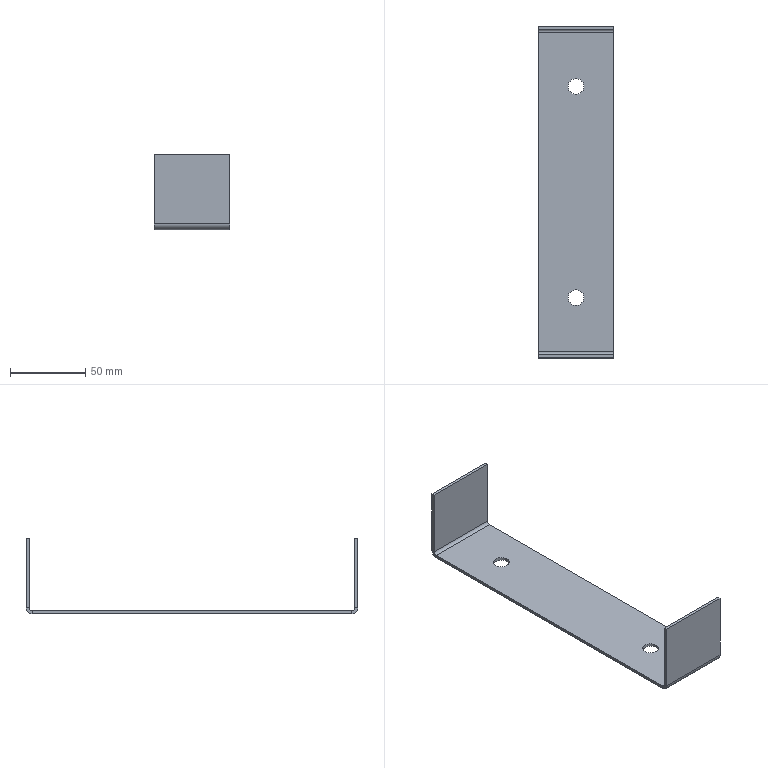Part | STEP file | SYL_0392D6J1SYL0380DJ100-674343 | 1 solid | 26 faces | box 50 x 220 x 50 mm | volume 30996 mm3 | plane 18 | cylinder 8 | commonest cylinder face diameters 10.5 x4 4 x2 8 x2
STEP:
#1=CARTESIAN_POINT('',(5.25,70.,-25.));
#2=VERTEX_POINT('',#1);
#3=CARTESIAN_POINT('',(5.25,70.,-23.));
#4=VERTEX_POINT('',#3);
#5=CARTESIAN_POINT('',(5.25,70.,-23.));
#6=DIRECTION('',(0.,0.,1.));
#7=VECTOR('',#6,1000.);
#8=LINE('',#5,#7);
#9=EDGE_CURVE('',#2,#4,#8,.T.);
#10=ORIENTED_EDGE('',*,*,#9,.F.);
#11=CARTESIAN_POINT('',(-5.25,70.,-25.));
#12=VERTEX_POINT('',#11);
#13=CARTESIAN_POINT('',(0.,70.,-25.));
#14=DIRECTION('',(0.,0.,-1.));
#15=DIRECTION('',(-1.,0.,0.));
#16=AXIS2_PLACEMENT_3D('',#13,#14,#15);
#17=CIRCLE('',#16,5.25);
#18=EDGE_CURVE('',#2,#12,#17,.T.);
#19=ORIENTED_EDGE('',*,*,#18,.T.);
#20=CARTESIAN_POINT('',(-5.25,70.,-23.));
#21=VERTEX_POINT('',#20);
#22=CARTESIAN_POINT('',(-5.25,70.,-23.));
#23=DIRECTION('',(0.,0.,1.));
#24=VECTOR('',#23,1000.);
#25=LINE('',#22,#24);
#26=EDGE_CURVE('',#12,#21,#25,.T.);
#27=ORIENTED_EDGE('',*,*,#26,.T.);
#28=CARTESIAN_POINT('',(0.,70.,-23.));
#29=DIRECTION('',(0.,0.,-1.));
#30=DIRECTION('',(1.,0.,0.));
#31=AXIS2_PLACEMENT_3D('',#28,#29,#30);
#32=CIRCLE('',#31,5.25);
#33=EDGE_CURVE('',#4,#21,#32,.T.);
#34=ORIENTED_EDGE('',*,*,#33,.F.);
#35=EDGE_LOOP('',(#10,#19,#27,#34));
#36=FACE_OUTER_BOUND('',#35,.T.);
#37=CARTESIAN_POINT('',(0.,70.,-23.));
#38=DIRECTION('',(0.,0.,-1.));
#39=DIRECTION('',(-1.,0.,0.));
#40=AXIS2_PLACEMENT_3D('',#37,#38,#39);
#41=CYLINDRICAL_SURFACE('',#40,5.25);
#42=ADVANCED_FACE('',(#36),#41,.F.);
#43=CARTESIAN_POINT('',(5.25,-70.,-25.));
#44=VERTEX_POINT('',#43);
#45=CARTESIAN_POINT('',(5.25,-70.,-23.));
#46=VERTEX_POINT('',#45);
#47=CARTESIAN_POINT('',(5.25,-70.,-23.));
#48=DIRECTION('',(0.,0.,1.));
#49=VECTOR('',#48,1000.);
#50=LINE('',#47,#49);
#51=EDGE_CURVE('',#44,#46,#50,.T.);
#52=ORIENTED_EDGE('',*,*,#51,.F.);
#53=CARTESIAN_POINT('',(-5.25,-70.,-25.));
#54=VERTEX_POINT('',#53);
#55=CARTESIAN_POINT('',(0.,-70.,-25.));
#56=DIRECTION('',(0.,0.,-1.));
#57=DIRECTION('',(-1.,0.,0.));
#58=AXIS2_PLACEMENT_3D('',#55,#56,#57);
#59=CIRCLE('',#58,5.25);
#60=EDGE_CURVE('',#44,#54,#59,.T.);
#61=ORIENTED_EDGE('',*,*,#60,.T.);
#62=CARTESIAN_POINT('',(-5.25,-70.,-23.));
#63=VERTEX_POINT('',#62);
#64=CARTESIAN_POINT('',(-5.25,-70.,-23.));
#65=DIRECTION('',(0.,0.,1.));
#66=VECTOR('',#65,1000.);
#67=LINE('',#64,#66);
#68=EDGE_CURVE('',#54,#63,#67,.T.);
#69=ORIENTED_EDGE('',*,*,#68,.T.);
#70=CARTESIAN_POINT('',(0.,-70.,-23.));
#71=DIRECTION('',(0.,0.,-1.));
#72=DIRECTION('',(1.,0.,0.));
#73=AXIS2_PLACEMENT_3D('',#70,#71,#72);
#74=CIRCLE('',#73,5.25);
#75=EDGE_CURVE('',#46,#63,#74,.T.);
#76=ORIENTED_EDGE('',*,*,#75,.F.);
#77=EDGE_LOOP('',(#52,#61,#69,#76));
#78=FACE_OUTER_BOUND('',#77,.T.);
#79=CARTESIAN_POINT('',(0.,-70.,-23.));
#80=DIRECTION('',(0.,0.,-1.));
#81=DIRECTION('',(-1.,0.,0.));
#82=AXIS2_PLACEMENT_3D('',#79,#80,#81);
#83=CYLINDRICAL_SURFACE('',#82,5.25);
#84=ADVANCED_FACE('',(#78),#83,.F.);
#85=CARTESIAN_POINT('',(25.,106.,-25.));
#86=VERTEX_POINT('',#85);
#87=CARTESIAN_POINT('',(25.,106.,-23.));
#88=VERTEX_POINT('',#87);
#89=CARTESIAN_POINT('',(25.,106.,-23.));
#90=DIRECTION('',(0.,0.,1.));
#91=VECTOR('',#90,1000.);
#92=LINE('',#89,#91);
#93=EDGE_CURVE('',#86,#88,#92,.T.);
#94=ORIENTED_EDGE('',*,*,#93,.F.);
#95=CARTESIAN_POINT('',(25.,110.,-21.));
#96=VERTEX_POINT('',#95);
#97=CARTESIAN_POINT('',(25.,106.,-21.));
#98=DIRECTION('',(-1.,0.,0.));
#99=DIRECTION('',(0.,0.,1.));
#100=AXIS2_PLACEMENT_3D('',#97,#98,#99);
#101=CIRCLE('',#100,4.);
#102=EDGE_CURVE('',#96,#86,#101,.T.);
#103=ORIENTED_EDGE('',*,*,#102,.F.);
#104=CARTESIAN_POINT('',(25.,108.,-21.));
#105=VERTEX_POINT('',#104);
#106=CARTESIAN_POINT('',(25.,108.,-21.));
#107=DIRECTION('',(0.,-1.,0.));
#108=VECTOR('',#107,1000.);
#109=LINE('',#106,#108);
#110=EDGE_CURVE('',#96,#105,#109,.T.);
#111=ORIENTED_EDGE('',*,*,#110,.T.);
#112=CARTESIAN_POINT('',(25.,106.,-21.));
#113=DIRECTION('',(-1.,0.,0.));
#114=DIRECTION('',(0.,1.,0.));
#115=AXIS2_PLACEMENT_3D('',#112,#113,#114);
#116=CIRCLE('',#115,2.);
#117=EDGE_CURVE('',#105,#88,#116,.T.);
#118=ORIENTED_EDGE('',*,*,#117,.T.);
#119=EDGE_LOOP('',(#94,#103,#111,#118));
#120=FACE_OUTER_BOUND('',#119,.T.);
#121=CARTESIAN_POINT('',(25.,106.,-21.));
#122=DIRECTION('',(1.,0.,0.));
#123=DIRECTION('',(0.,0.,-1.));
#124=AXIS2_PLACEMENT_3D('',#121,#122,#123);
#125=PLANE('',#124);
#126=ADVANCED_FACE('',(#120),#125,.T.);
#127=ORIENTED_EDGE('',*,*,#110,.F.);
#128=CARTESIAN_POINT('',(25.,110.,25.));
#129=VERTEX_POINT('',#128);
#130=CARTESIAN_POINT('',(25.,110.,-25.));
#131=DIRECTION('',(0.,0.,-1.));
#132=VECTOR('',#131,1000.);
#133=LINE('',#130,#132);
#134=EDGE_CURVE('',#129,#96,#133,.T.);
#135=ORIENTED_EDGE('',*,*,#134,.F.);
#136=CARTESIAN_POINT('',(25.,108.,25.));
#137=VERTEX_POINT('',#136);
#138=CARTESIAN_POINT('',(25.,108.,25.));
#139=DIRECTION('',(0.,-1.,0.));
#140=VECTOR('',#139,1000.);
#141=LINE('',#138,#140);
#142=EDGE_CURVE('',#129,#137,#141,.T.);
#143=ORIENTED_EDGE('',*,*,#142,.T.);
#144=CARTESIAN_POINT('',(25.,108.,25.));
#145=DIRECTION('',(0.,0.,-1.));
#146=VECTOR('',#145,1000.);
#147=LINE('',#144,#146);
#148=EDGE_CURVE('',#137,#105,#147,.T.);
#149=ORIENTED_EDGE('',*,*,#148,.T.);
#150=EDGE_LOOP('',(#127,#135,#143,#149));
#151=FACE_OUTER_BOUND('',#150,.T.);
#152=CARTESIAN_POINT('',(25.,108.,25.));
#153=DIRECTION('',(1.,0.,0.));
#154=DIRECTION('',(0.,0.,-1.));
#155=AXIS2_PLACEMENT_3D('',#152,#153,#154);
#156=PLANE('',#155);
#157=ADVANCED_FACE('',(#151),#156,.T.);
#158=ORIENTED_EDGE('',*,*,#142,.F.);
#159=CARTESIAN_POINT('',(-25.,110.,25.));
#160=VERTEX_POINT('',#159);
#161=CARTESIAN_POINT('',(-25.,110.,25.));
#162=DIRECTION('',(-1.,0.,0.));
#163=VECTOR('',#162,1000.);
#164=LINE('',#161,#163);
#165=EDGE_CURVE('',#129,#160,#164,.T.);
#166=ORIENTED_EDGE('',*,*,#165,.T.);
#167=CARTESIAN_POINT('',(-25.,108.,25.));
#168=VERTEX_POINT('',#167);
#169=CARTESIAN_POINT('',(-25.,108.,25.));
#170=DIRECTION('',(0.,-1.,0.));
#171=VECTOR('',#170,1000.);
#172=LINE('',#169,#171);
#173=EDGE_CURVE('',#160,#168,#172,.T.);
#174=ORIENTED_EDGE('',*,*,#173,.T.);
#175=CARTESIAN_POINT('',(25.,108.,25.));
#176=DIRECTION('',(-1.,0.,0.));
#177=VECTOR('',#176,1000.);
#178=LINE('',#175,#177);
#179=EDGE_CURVE('',#137,#168,#178,.T.);
#180=ORIENTED_EDGE('',*,*,#179,.F.);
#181=EDGE_LOOP('',(#158,#166,#174,#180));
#182=FACE_OUTER_BOUND('',#181,.T.);
#183=CARTESIAN_POINT('',(25.,108.,25.));
#184=DIRECTION('',(0.,0.,-1.));
#185=DIRECTION('',(-1.,0.,0.));
#186=AXIS2_PLACEMENT_3D('',#183,#184,#185);
#187=PLANE('',#186);
#188=ADVANCED_FACE('',(#182),#187,.F.);
#189=ORIENTED_EDGE('',*,*,#173,.F.);
#190=CARTESIAN_POINT('',(-25.,110.,-21.));
#191=VERTEX_POINT('',#190);
#192=CARTESIAN_POINT('',(-25.,110.,-25.));
#193=DIRECTION('',(0.,0.,-1.));
#194=VECTOR('',#193,1000.);
#195=LINE('',#192,#194);
#196=EDGE_CURVE('',#160,#191,#195,.T.);
#197=ORIENTED_EDGE('',*,*,#196,.T.);
#198=CARTESIAN_POINT('',(-25.,108.,-21.));
#199=VERTEX_POINT('',#198);
#200=CARTESIAN_POINT('',(-25.,108.,-21.));
#201=DIRECTION('',(0.,-1.,0.));
#202=VECTOR('',#201,1000.);
#203=LINE('',#200,#202);
#204=EDGE_CURVE('',#191,#199,#203,.T.);
#205=ORIENTED_EDGE('',*,*,#204,.T.);
#206=CARTESIAN_POINT('',(-25.,108.,25.));
#207=DIRECTION('',(0.,0.,-1.));
#208=VECTOR('',#207,1000.);
#209=LINE('',#206,#208);
#210=EDGE_CURVE('',#168,#199,#209,.T.);
#211=ORIENTED_EDGE('',*,*,#210,.F.);
#212=EDGE_LOOP('',(#189,#197,#205,#211));
#213=FACE_OUTER_BOUND('',#212,.T.);
#214=CARTESIAN_POINT('',(-25.,108.,25.));
#215=DIRECTION('',(1.,0.,0.));
#216=DIRECTION('',(0.,0.,-1.));
#217=AXIS2_PLACEMENT_3D('',#214,#215,#216);
#218=PLANE('',#217);
#219=ADVANCED_FACE('',(#213),#218,.F.);
#220=ORIENTED_EDGE('',*,*,#204,.F.);
#221=CARTESIAN_POINT('',(-25.,106.,-25.));
#222=VERTEX_POINT('',#221);
#223=CARTESIAN_POINT('',(-25.,106.,-21.));
#224=DIRECTION('',(1.,0.,0.));
#225=DIRECTION('',(0.,0.,1.));
#226=AXIS2_PLACEMENT_3D('',#223,#224,#225);
#227=CIRCLE('',#226,4.);
#228=EDGE_CURVE('',#222,#191,#227,.T.);
#229=ORIENTED_EDGE('',*,*,#228,.F.);
#230=CARTESIAN_POINT('',(-25.,106.,-23.));
#231=VERTEX_POINT('',#230);
#232=CARTESIAN_POINT('',(-25.,106.,-23.));
#233=DIRECTION('',(0.,0.,1.));
#234=VECTOR('',#233,1000.);
#235=LINE('',#232,#234);
#236=EDGE_CURVE('',#222,#231,#235,.T.);
#237=ORIENTED_EDGE('',*,*,#236,.T.);
#238=CARTESIAN_POINT('',(-25.,106.,-21.));
#239=DIRECTION('',(1.,0.,0.));
#240=DIRECTION('',(0.,0.,-1.));
#241=AXIS2_PLACEMENT_3D('',#238,#239,#240);
#242=CIRCLE('',#241,2.);
#243=EDGE_CURVE('',#231,#199,#242,.T.);
#244=ORIENTED_EDGE('',*,*,#243,.T.);
#245=EDGE_LOOP('',(#220,#229,#237,#244));
#246=FACE_OUTER_BOUND('',#245,.T.);
#247=CARTESIAN_POINT('',(-25.,106.,-21.));
#248=DIRECTION('',(-1.,0.,0.));
#249=DIRECTION('',(0.,0.,1.));
#250=AXIS2_PLACEMENT_3D('',#247,#248,#249);
#251=PLANE('',#250);
#252=ADVANCED_FACE('',(#246),#251,.T.);
#253=ORIENTED_EDGE('',*,*,#236,.F.);
#254=CARTESIAN_POINT('',(-25.,-106.,-25.));
#255=VERTEX_POINT('',#254);
#256=CARTESIAN_POINT('',(-25.,-110.,-25.));
#257=DIRECTION('',(0.,-1.,0.));
#258=VECTOR('',#257,1000.);
#259=LINE('',#256,#258);
#260=EDGE_CURVE('',#222,#255,#259,.T.);
#261=ORIENTED_EDGE('',*,*,#260,.T.);
#262=CARTESIAN_POINT('',(-25.,-106.,-23.));
#263=VERTEX_POINT('',#262);
#264=CARTESIAN_POINT('',(-25.,-106.,-23.));
#265=DIRECTION('',(0.,0.,1.));
#266=VECTOR('',#265,1000.);
#267=LINE('',#264,#266);
#268=EDGE_CURVE('',#255,#263,#267,.T.);
#269=ORIENTED_EDGE('',*,*,#268,.T.);
#270=CARTESIAN_POINT('',(-25.,106.,-23.));
#271=DIRECTION('',(0.,-1.,0.));
#272=VECTOR('',#271,1000.);
#273=LINE('',#270,#272);
#274=EDGE_CURVE('',#231,#263,#273,.T.);
#275=ORIENTED_EDGE('',*,*,#274,.F.);
#276=EDGE_LOOP('',(#253,#261,#269,#275));
#277=FACE_OUTER_BOUND('',#276,.T.);
#278=CARTESIAN_POINT('',(-25.,106.,-23.));
#279=DIRECTION('',(1.,0.,0.));
#280=DIRECTION('',(0.,-1.,0.));
#281=AXIS2_PLACEMENT_3D('',#278,#279,#280);
#282=PLANE('',#281);
#283=ADVANCED_FACE('',(#277),#282,.F.);
#284=ORIENTED_EDGE('',*,*,#268,.F.);
#285=CARTESIAN_POINT('',(-25.,-110.,-21.));
#286=VERTEX_POINT('',#285);
#287=CARTESIAN_POINT('',(-25.,-106.,-21.));
#288=DIRECTION('',(1.,0.,0.));
#289=DIRECTION('',(0.,0.,1.));
#290=AXIS2_PLACEMENT_3D('',#287,#288,#289);
#291=CIRCLE('',#290,4.);
#292=EDGE_CURVE('',#286,#255,#291,.T.);
#293=ORIENTED_EDGE('',*,*,#292,.F.);
#294=CARTESIAN_POINT('',(-25.,-108.,-21.));
#295=VERTEX_POINT('',#294);
#296=CARTESIAN_POINT('',(-25.,-108.,-21.));
#297=DIRECTION('',(0.,1.,0.));
#298=VECTOR('',#297,1000.);
#299=LINE('',#296,#298);
#300=EDGE_CURVE('',#286,#295,#299,.T.);
#301=ORIENTED_EDGE('',*,*,#300,.T.);
#302=CARTESIAN_POINT('',(-25.,-106.,-21.));
#303=DIRECTION('',(1.,0.,0.));
#304=DIRECTION('',(0.,-1.,0.));
#305=AXIS2_PLACEMENT_3D('',#302,#303,#304);
#306=CIRCLE('',#305,2.);
#307=EDGE_CURVE('',#295,#263,#306,.T.);
#308=ORIENTED_EDGE('',*,*,#307,.T.);
#309=EDGE_LOOP('',(#284,#293,#301,#308));
#310=FACE_OUTER_BOUND('',#309,.T.);
#311=CARTESIAN_POINT('',(-25.,-106.,-21.));
#312=DIRECTION('',(-1.,0.,0.));
#313=DIRECTION('',(0.,0.,1.));
#314=AXIS2_PLACEMENT_3D('',#311,#312,#313);
#315=PLANE('',#314);
#316=ADVANCED_FACE('',(#310),#315,.T.);
#317=ORIENTED_EDGE('',*,*,#300,.F.);
#318=CARTESIAN_POINT('',(-25.,-110.,25.));
#319=VERTEX_POINT('',#318);
#320=CARTESIAN_POINT('',(-25.,-110.,25.));
#321=DIRECTION('',(0.,0.,1.));
#322=VECTOR('',#321,1000.);
#323=LINE('',#320,#322);
#324=EDGE_CURVE('',#286,#319,#323,.T.);
#325=ORIENTED_EDGE('',*,*,#324,.T.);
#326=CARTESIAN_POINT('',(-25.,-108.,25.));
#327=VERTEX_POINT('',#326);
#328=CARTESIAN_POINT('',(-25.,-108.,25.));
#329=DIRECTION('',(0.,1.,0.));
#330=VECTOR('',#329,1000.);
#331=LINE('',#328,#330);
#332=EDGE_CURVE('',#319,#327,#331,.T.);
#333=ORIENTED_EDGE('',*,*,#332,.T.);
#334=CARTESIAN_POINT('',(-25.,-108.,-21.));
#335=DIRECTION('',(0.,0.,1.));
#336=VECTOR('',#335,1000.);
#337=LINE('',#334,#336);
#338=EDGE_CURVE('',#295,#327,#337,.T.);
#339=ORIENTED_EDGE('',*,*,#338,.F.);
#340=EDGE_LOOP('',(#317,#325,#333,#339));
#341=FACE_OUTER_BOUND('',#340,.T.);
#342=CARTESIAN_POINT('',(-25.,-108.,-21.));
#343=DIRECTION('',(1.,0.,0.));
#344=DIRECTION('',(0.,0.,1.));
#345=AXIS2_PLACEMENT_3D('',#342,#343,#344);
#346=PLANE('',#345);
#347=ADVANCED_FACE('',(#341),#346,.F.);
#348=ORIENTED_EDGE('',*,*,#332,.F.);
#349=CARTESIAN_POINT('',(25.,-110.,25.));
#350=VERTEX_POINT('',#349);
#351=CARTESIAN_POINT('',(-25.,-110.,25.));
#352=DIRECTION('',(-1.,0.,0.));
#353=VECTOR('',#352,1000.);
#354=LINE('',#351,#353);
#355=EDGE_CURVE('',#350,#319,#354,.T.);
#356=ORIENTED_EDGE('',*,*,#355,.F.);
#357=CARTESIAN_POINT('',(25.,-108.,25.));
#358=VERTEX_POINT('',#357);
#359=CARTESIAN_POINT('',(25.,-108.,25.));
#360=DIRECTION('',(0.,1.,0.));
#361=VECTOR('',#360,1000.);
#362=LINE('',#359,#361);
#363=EDGE_CURVE('',#350,#358,#362,.T.);
#364=ORIENTED_EDGE('',*,*,#363,.T.);
#365=CARTESIAN_POINT('',(25.,-108.,25.));
#366=DIRECTION('',(-1.,0.,0.));
#367=VECTOR('',#366,1000.);
#368=LINE('',#365,#367);
#369=EDGE_CURVE('',#358,#327,#368,.T.);
#370=ORIENTED_EDGE('',*,*,#369,.T.);
#371=EDGE_LOOP('',(#348,#356,#364,#370));
#372=FACE_OUTER_BOUND('',#371,.T.);
#373=CARTESIAN_POINT('',(25.,-108.,25.));
#374=DIRECTION('',(0.,0.,1.));
#375=DIRECTION('',(-1.,0.,0.));
#376=AXIS2_PLACEMENT_3D('',#373,#374,#375);
#377=PLANE('',#376);
#378=ADVANCED_FACE('',(#372),#377,.T.);
#379=ORIENTED_EDGE('',*,*,#363,.F.);
#380=CARTESIAN_POINT('',(25.,-110.,-21.));
#381=VERTEX_POINT('',#380);
#382=CARTESIAN_POINT('',(25.,-110.,25.));
#383=DIRECTION('',(0.,0.,1.));
#384=VECTOR('',#383,1000.);
#385=LINE('',#382,#384);
#386=EDGE_CURVE('',#381,#350,#385,.T.);
#387=ORIENTED_EDGE('',*,*,#386,.F.);
#388=CARTESIAN_POINT('',(25.,-108.,-21.));
#389=VERTEX_POINT('',#388);
#390=CARTESIAN_POINT('',(25.,-108.,-21.));
#391=DIRECTION('',(0.,1.,0.));
#392=VECTOR('',#391,1000.);
#393=LINE('',#390,#392);
#394=EDGE_CURVE('',#381,#389,#393,.T.);
#395=ORIENTED_EDGE('',*,*,#394,.T.);
#396=CARTESIAN_POINT('',(25.,-108.,-21.));
#397=DIRECTION('',(0.,0.,1.));
#398=VECTOR('',#397,1000.);
#399=LINE('',#396,#398);
#400=EDGE_CURVE('',#389,#358,#399,.T.);
#401=ORIENTED_EDGE('',*,*,#400,.T.);
#402=EDGE_LOOP('',(#379,#387,#395,#401));
#403=FACE_OUTER_BOUND('',#402,.T.);
#404=CARTESIAN_POINT('',(25.,-108.,-21.));
#405=DIRECTION('',(1.,0.,0.));
#406=DIRECTION('',(0.,0.,1.));
#407=AXIS2_PLACEMENT_3D('',#404,#405,#406);
#408=PLANE('',#407);
#409=ADVANCED_FACE('',(#403),#408,.T.);
#410=ORIENTED_EDGE('',*,*,#394,.F.);
#411=CARTESIAN_POINT('',(25.,-106.,-25.));
#412=VERTEX_POINT('',#411);
#413=CARTESIAN_POINT('',(25.,-106.,-21.));
#414=DIRECTION('',(-1.,0.,0.));
#415=DIRECTION('',(0.,0.,1.));
#416=AXIS2_PLACEMENT_3D('',#413,#414,#415);
#417=CIRCLE('',#416,4.);
#418=EDGE_CURVE('',#412,#381,#417,.T.);
#419=ORIENTED_EDGE('',*,*,#418,.F.);
#420=CARTESIAN_POINT('',(25.,-106.,-23.));
#421=VERTEX_POINT('',#420);
#422=CARTESIAN_POINT('',(25.,-106.,-23.));
#423=DIRECTION('',(0.,0.,1.));
#424=VECTOR('',#423,1000.);
#425=LINE('',#422,#424);
#426=EDGE_CURVE('',#412,#421,#425,.T.);
#427=ORIENTED_EDGE('',*,*,#426,.T.);
#428=CARTESIAN_POINT('',(25.,-106.,-21.));
#429=DIRECTION('',(-1.,0.,0.));
#430=DIRECTION('',(0.,0.,-1.));
#431=AXIS2_PLACEMENT_3D('',#428,#429,#430);
#432=CIRCLE('',#431,2.);
#433=EDGE_CURVE('',#421,#389,#432,.T.);
#434=ORIENTED_EDGE('',*,*,#433,.T.);
#435=EDGE_LOOP('',(#410,#419,#427,#434));
#436=FACE_OUTER_BOUND('',#435,.T.);
#437=CARTESIAN_POINT('',(25.,-106.,-21.));
#438=DIRECTION('',(1.,0.,0.));
#439=DIRECTION('',(0.,0.,-1.));
#440=AXIS2_PLACEMENT_3D('',#437,#438,#439);
#441=PLANE('',#440);
#442=ADVANCED_FACE('',(#436),#441,.T.);
#443=CARTESIAN_POINT('',(0.,-70.,-25.));
#444=DIRECTION('',(0.,0.,-1.));
#445=DIRECTION('',(-1.,0.,0.));
#446=AXIS2_PLACEMENT_3D('',#443,#444,#445);
#447=CIRCLE('',#446,5.25);
#448=EDGE_CURVE('',#54,#44,#447,.T.);
#449=ORIENTED_EDGE('',*,*,#448,.T.);
#450=ORIENTED_EDGE('',*,*,#51,.T.);
#451=CARTESIAN_POINT('',(0.,-70.,-23.));
#452=DIRECTION('',(0.,0.,-1.));
#453=DIRECTION('',(-1.,0.,0.));
#454=AXIS2_PLACEMENT_3D('',#451,#452,#453);
#455=CIRCLE('',#454,5.25);
#456=EDGE_CURVE('',#63,#46,#455,.T.);
#457=ORIENTED_EDGE('',*,*,#456,.F.);
#458=ORIENTED_EDGE('',*,*,#68,.F.);
#459=EDGE_LOOP('',(#449,#450,#457,#458));
#460=FACE_OUTER_BOUND('',#459,.T.);
#461=CARTESIAN_POINT('',(0.,-70.,-23.));
#462=DIRECTION('',(0.,0.,-1.));
#463=DIRECTION('',(-1.,0.,0.));
#464=AXIS2_PLACEMENT_3D('',#461,#462,#463);
#465=CYLINDRICAL_SURFACE('',#464,5.25);
#466=ADVANCED_FACE('',(#460),#465,.F.);
#467=CARTESIAN_POINT('',(0.,70.,-25.));
#468=DIRECTION('',(0.,0.,-1.));
#469=DIRECTION('',(-1.,0.,0.));
#470=AXIS2_PLACEMENT_3D('',#467,#468,#469);
#471=CIRCLE('',#470,5.25);
#472=EDGE_CURVE('',#12,#2,#471,.T.);
#473=ORIENTED_EDGE('',*,*,#472,.T.);
#474=ORIENTED_EDGE('',*,*,#9,.T.);
#475=CARTESIAN_POINT('',(0.,70.,-23.));
#476=DIRECTION('',(0.,0.,-1.));
#477=DIRECTION('',(-1.,0.,0.));
#478=AXIS2_PLACEMENT_3D('',#475,#476,#477);
#479=CIRCLE('',#478,5.25);
#480=EDGE_CURVE('',#21,#4,#479,.T.);
#481=ORIENTED_EDGE('',*,*,#480,.F.);
#482=ORIENTED_EDGE('',*,*,#26,.F.);
#483=EDGE_LOOP('',(#473,#474,#481,#482));
#484=FACE_OUTER_BOUND('',#483,.T.);
#485=CARTESIAN_POINT('',(0.,70.,-23.));
#486=DIRECTION('',(0.,0.,-1.));
#487=DIRECTION('',(-1.,0.,0.));
#488=AXIS2_PLACEMENT_3D('',#485,#486,#487);
#489=CYLINDRICAL_SURFACE('',#488,5.25);
#490=ADVANCED_FACE('',(#484),#489,.F.);
#491=CARTESIAN_POINT('',(25.,-110.,-25.));
#492=DIRECTION('',(0.,-1.,0.));
#493=VECTOR('',#492,1000.);
#494=LINE('',#491,#493);
#495=EDGE_CURVE('',#86,#412,#494,.T.);
#496=ORIENTED_EDGE('',*,*,#495,.F.);
#497=ORIENTED_EDGE('',*,*,#93,.T.);
#498=CARTESIAN_POINT('',(25.,106.,-23.));
#499=DIRECTION('',(0.,-1.,0.));
#500=VECTOR('',#499,1000.);
#501=LINE('',#498,#500);
#502=EDGE_CURVE('',#88,#421,#501,.T.);
#503=ORIENTED_EDGE('',*,*,#502,.T.);
#504=ORIENTED_EDGE('',*,*,#426,.F.);
#505=EDGE_LOOP('',(#496,#497,#503,#504));
#506=FACE_OUTER_BOUND('',#505,.T.);
#507=CARTESIAN_POINT('',(25.,106.,-23.));
#508=DIRECTION('',(1.,0.,0.));
#509=DIRECTION('',(0.,-1.,0.));
#510=AXIS2_PLACEMENT_3D('',#507,#508,#509);
#511=PLANE('',#510);
#512=ADVANCED_FACE('',(#506),#511,.T.);
#513=ORIENTED_EDGE('',*,*,#433,.F.);
#514=CARTESIAN_POINT('',(25.,-106.,-23.));
#515=DIRECTION('',(-1.,0.,0.));
#516=VECTOR('',#515,1000.);
#517=LINE('',#514,#516);
#518=EDGE_CURVE('',#421,#263,#517,.T.);
#519=ORIENTED_EDGE('',*,*,#518,.T.);
#520=ORIENTED_EDGE('',*,*,#307,.F.);
#521=CARTESIAN_POINT('',(-25.,-108.,-21.));
#522=DIRECTION('',(1.,0.,0.));
#523=VECTOR('',#522,1000.);
#524=LINE('',#521,#523);
#525=EDGE_CURVE('',#295,#389,#524,.T.);
#526=ORIENTED_EDGE('',*,*,#525,.T.);
#527=EDGE_LOOP('',(#513,#519,#520,#526));
#528=FACE_OUTER_BOUND('',#527,.T.);
#529=CARTESIAN_POINT('',(-25.,-106.,-21.));
#530=DIRECTION('',(-1.,0.,0.));
#531=DIRECTION('',(0.,0.,1.));
#532=AXIS2_PLACEMENT_3D('',#529,#530,#531);
#533=CYLINDRICAL_SURFACE('',#532,2.);
#534=ADVANCED_FACE('',(#528),#533,.F.);
#535=ORIENTED_EDGE('',*,*,#525,.F.);
#536=ORIENTED_EDGE('',*,*,#338,.T.);
#537=ORIENTED_EDGE('',*,*,#369,.F.);
#538=ORIENTED_EDGE('',*,*,#400,.F.);
#539=EDGE_LOOP('',(#535,#536,#537,#538));
#540=FACE_OUTER_BOUND('',#539,.T.);
#541=CARTESIAN_POINT('',(-25.,-108.,25.));
#542=DIRECTION('',(0.,-1.,0.));
#543=DIRECTION('',(0.,0.,-1.));
#544=AXIS2_PLACEMENT_3D('',#541,#542,#543);
#545=PLANE('',#544);
#546=ADVANCED_FACE('',(#540),#545,.F.);
#547=ORIENTED_EDGE('',*,*,#117,.F.);
#548=CARTESIAN_POINT('',(25.,108.,-21.));
#549=DIRECTION('',(-1.,0.,0.));
#550=VECTOR('',#549,1000.);
#551=LINE('',#548,#550);
#552=EDGE_CURVE('',#105,#199,#551,.T.);
#553=ORIENTED_EDGE('',*,*,#552,.T.);
#554=ORIENTED_EDGE('',*,*,#243,.F.);
#555=CARTESIAN_POINT('',(-25.,106.,-23.));
#556=DIRECTION('',(1.,0.,0.));
#557=VECTOR('',#556,1000.);
#558=LINE('',#555,#557);
#559=EDGE_CURVE('',#231,#88,#558,.T.);
#560=ORIENTED_EDGE('',*,*,#559,.T.);
#561=EDGE_LOOP('',(#547,#553,#554,#560));
#562=FACE_OUTER_BOUND('',#561,.T.);
#563=CARTESIAN_POINT('',(-25.,106.,-21.));
#564=DIRECTION('',(-1.,0.,0.));
#565=DIRECTION('',(0.,0.,1.));
#566=AXIS2_PLACEMENT_3D('',#563,#564,#565);
#567=CYLINDRICAL_SURFACE('',#566,2.);
#568=ADVANCED_FACE('',(#562),#567,.F.);
#569=ORIENTED_EDGE('',*,*,#75,.T.);
#570=ORIENTED_EDGE('',*,*,#456,.T.);
#571=EDGE_LOOP('',(#569,#570));
#572=FACE_BOUND('',#571,.T.);
#573=ORIENTED_EDGE('',*,*,#33,.T.);
#574=ORIENTED_EDGE('',*,*,#480,.T.);
#575=EDGE_LOOP('',(#573,#574));
#576=FACE_BOUND('',#575,.T.);
#577=ORIENTED_EDGE('',*,*,#559,.F.);
#578=ORIENTED_EDGE('',*,*,#274,.T.);
#579=ORIENTED_EDGE('',*,*,#518,.F.);
#580=ORIENTED_EDGE('',*,*,#502,.F.);
#581=EDGE_LOOP('',(#577,#578,#579,#580));
#582=FACE_OUTER_BOUND('',#581,.T.);
#583=CARTESIAN_POINT('',(-25.,-110.,-23.));
#584=DIRECTION('',(0.,0.,-1.));
#585=DIRECTION('',(0.,-1.,0.));
#586=AXIS2_PLACEMENT_3D('',#583,#584,#585);
#587=PLANE('',#586);
#588=ADVANCED_FACE('',(#572,#576,#582),#587,.F.);
#589=ORIENTED_EDGE('',*,*,#179,.T.);
#590=ORIENTED_EDGE('',*,*,#210,.T.);
#591=ORIENTED_EDGE('',*,*,#552,.F.);
#592=ORIENTED_EDGE('',*,*,#148,.F.);
#593=EDGE_LOOP('',(#589,#590,#591,#592));
#594=FACE_OUTER_BOUND('',#593,.T.);
#595=CARTESIAN_POINT('',(-25.,108.,-25.));
#596=DIRECTION('',(0.,1.,0.));
#597=DIRECTION('',(1.,0.,0.));
#598=AXIS2_PLACEMENT_3D('',#595,#596,#597);
#599=PLANE('',#598);
#600=ADVANCED_FACE('',(#594),#599,.F.);
#601=ORIENTED_EDGE('',*,*,#418,.T.);
#602=CARTESIAN_POINT('',(-25.,-110.,-21.));
#603=DIRECTION('',(1.,0.,0.));
#604=VECTOR('',#603,1000.);
#605=LINE('',#602,#604);
#606=EDGE_CURVE('',#286,#381,#605,.T.);
#607=ORIENTED_EDGE('',*,*,#606,.F.);
#608=ORIENTED_EDGE('',*,*,#292,.T.);
#609=CARTESIAN_POINT('',(-25.,-106.,-25.));
#610=DIRECTION('',(-1.,0.,0.));
#611=VECTOR('',#610,1000.);
#612=LINE('',#609,#611);
#613=EDGE_CURVE('',#412,#255,#612,.T.);
#614=ORIENTED_EDGE('',*,*,#613,.F.);
#615=EDGE_LOOP('',(#601,#607,#608,#614));
#616=FACE_OUTER_BOUND('',#615,.T.);
#617=CARTESIAN_POINT('',(-25.,-106.,-21.));
#618=DIRECTION('',(-1.,0.,0.));
#619=DIRECTION('',(0.,0.,1.));
#620=AXIS2_PLACEMENT_3D('',#617,#618,#619);
#621=CYLINDRICAL_SURFACE('',#620,4.);
#622=ADVANCED_FACE('',(#616),#621,.T.);
#623=ORIENTED_EDGE('',*,*,#606,.T.);
#624=ORIENTED_EDGE('',*,*,#386,.T.);
#625=ORIENTED_EDGE('',*,*,#355,.T.);
#626=ORIENTED_EDGE('',*,*,#324,.F.);
#627=EDGE_LOOP('',(#623,#624,#625,#626));
#628=FACE_OUTER_BOUND('',#627,.T.);
#629=CARTESIAN_POINT('',(-25.,-110.,25.));
#630=DIRECTION('',(0.,-1.,0.));
#631=DIRECTION('',(0.,0.,-1.));
#632=AXIS2_PLACEMENT_3D('',#629,#630,#631);
#633=PLANE('',#632);
#634=ADVANCED_FACE('',(#628),#633,.T.);
#635=ORIENTED_EDGE('',*,*,#102,.T.);
#636=CARTESIAN_POINT('',(-25.,106.,-25.));
#637=DIRECTION('',(1.,0.,0.));
#638=VECTOR('',#637,1000.);
#639=LINE('',#636,#638);
#640=EDGE_CURVE('',#222,#86,#639,.T.);
#641=ORIENTED_EDGE('',*,*,#640,.F.);
#642=ORIENTED_EDGE('',*,*,#228,.T.);
#643=CARTESIAN_POINT('',(-25.,110.,-21.));
#644=DIRECTION('',(-1.,0.,0.));
#645=VECTOR('',#644,1000.);
#646=LINE('',#643,#645);
#647=EDGE_CURVE('',#96,#191,#646,.T.);
#648=ORIENTED_EDGE('',*,*,#647,.F.);
#649=EDGE_LOOP('',(#635,#641,#642,#648));
#650=FACE_OUTER_BOUND('',#649,.T.);
#651=CARTESIAN_POINT('',(-25.,106.,-21.));
#652=DIRECTION('',(-1.,0.,0.));
#653=DIRECTION('',(0.,0.,1.));
#654=AXIS2_PLACEMENT_3D('',#651,#652,#653);
#655=CYLINDRICAL_SURFACE('',#654,4.);
#656=ADVANCED_FACE('',(#650),#655,.T.);
#657=ORIENTED_EDGE('',*,*,#60,.F.);
#658=ORIENTED_EDGE('',*,*,#448,.F.);
#659=EDGE_LOOP('',(#657,#658));
#660=FACE_BOUND('',#659,.T.);
#661=ORIENTED_EDGE('',*,*,#18,.F.);
#662=ORIENTED_EDGE('',*,*,#472,.F.);
#663=EDGE_LOOP('',(#661,#662));
#664=FACE_BOUND('',#663,.T.);
#665=ORIENTED_EDGE('',*,*,#640,.T.);
#666=ORIENTED_EDGE('',*,*,#495,.T.);
#667=ORIENTED_EDGE('',*,*,#613,.T.);
#668=ORIENTED_EDGE('',*,*,#260,.F.);
#669=EDGE_LOOP('',(#665,#666,#667,#668));
#670=FACE_OUTER_BOUND('',#669,.T.);
#671=CARTESIAN_POINT('',(-25.,-110.,-25.));
#672=DIRECTION('',(0.,0.,-1.));
#673=DIRECTION('',(0.,-1.,0.));
#674=AXIS2_PLACEMENT_3D('',#671,#672,#673);
#675=PLANE('',#674);
#676=ADVANCED_FACE('',(#660,#664,#670),#675,.T.);
#677=ORIENTED_EDGE('',*,*,#165,.F.);
#678=ORIENTED_EDGE('',*,*,#134,.T.);
#679=ORIENTED_EDGE('',*,*,#647,.T.);
#680=ORIENTED_EDGE('',*,*,#196,.F.);
#681=EDGE_LOOP('',(#677,#678,#679,#680));
#682=FACE_OUTER_BOUND('',#681,.T.);
#683=CARTESIAN_POINT('',(-25.,110.,-25.));
#684=DIRECTION('',(0.,1.,0.));
#685=DIRECTION('',(1.,0.,0.));
#686=AXIS2_PLACEMENT_3D('',#683,#684,#685);
#687=PLANE('',#686);
#688=ADVANCED_FACE('',(#682),#687,.T.);
#689=CLOSED_SHELL('',(#42,#84,#126,#157,#188,#219,#252,#283,#316,#347,#378,#409,#442,#466,#490,#512,#534,#546,#568,#588,#600,#622,#634,#656,#676,#688));
#690=MANIFOLD_SOLID_BREP('',#689);
#691=CARTESIAN_POINT('',(0.,0.,0.));
#692=DIRECTION('',(0.,0.,1.));
#693=DIRECTION('',(1.,0.,0.));
#694=AXIS2_PLACEMENT_3D('',#691,#692,#693);
#695=(LENGTH_UNIT()NAMED_UNIT(*)SI_UNIT(.MILLI.,.METRE.));
#696=UNCERTAINTY_MEASURE_WITH_UNIT(LENGTH_MEASURE(0.00001),#695,'','');
#697=(NAMED_UNIT(*)PLANE_ANGLE_UNIT()SI_UNIT($,.RADIAN.));
#698=(NAMED_UNIT(*)SI_UNIT($,.STERADIAN.)SOLID_ANGLE_UNIT());
#699=(GEOMETRIC_REPRESENTATION_CONTEXT(3)GLOBAL_UNCERTAINTY_ASSIGNED_CONTEXT((#696))GLOBAL_UNIT_ASSIGNED_CONTEXT((#695,#697,#698))REPRESENTATION_CONTEXT('',''));
#700=ADVANCED_BREP_SHAPE_REPRESENTATION('',(#690,#694),#699);